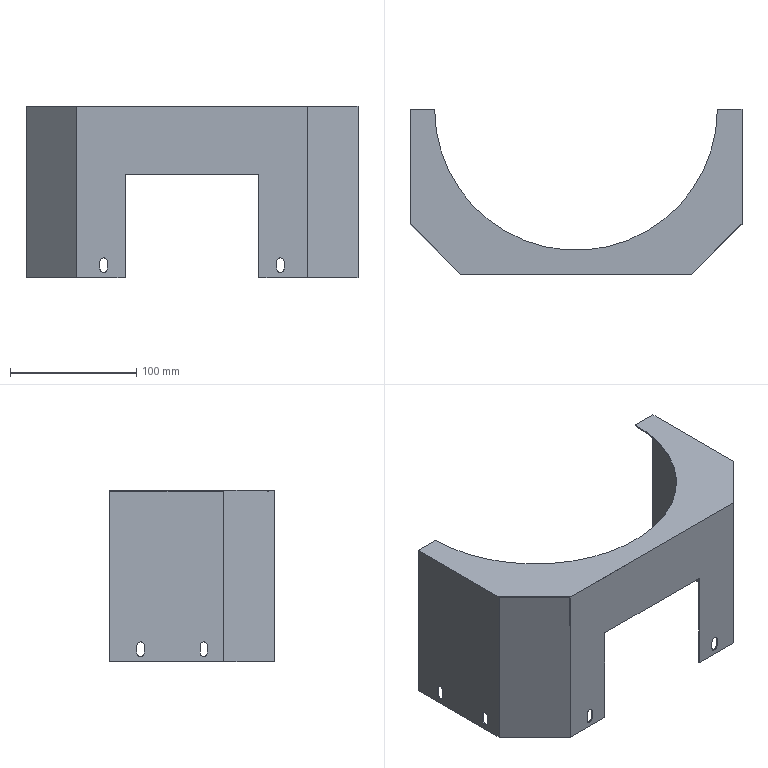Part | SolidWorks | features Cut 2, HoleWzd 2, Chamfer 1, Extrusion 1, Shell 1 | 1 solid | 50 faces | box 263 x 130.5 x 136 mm | volume 68260 mm3 | plane 31 | cylinder 19 | commonest cylinder face diameters 5.8 x18 224 x1